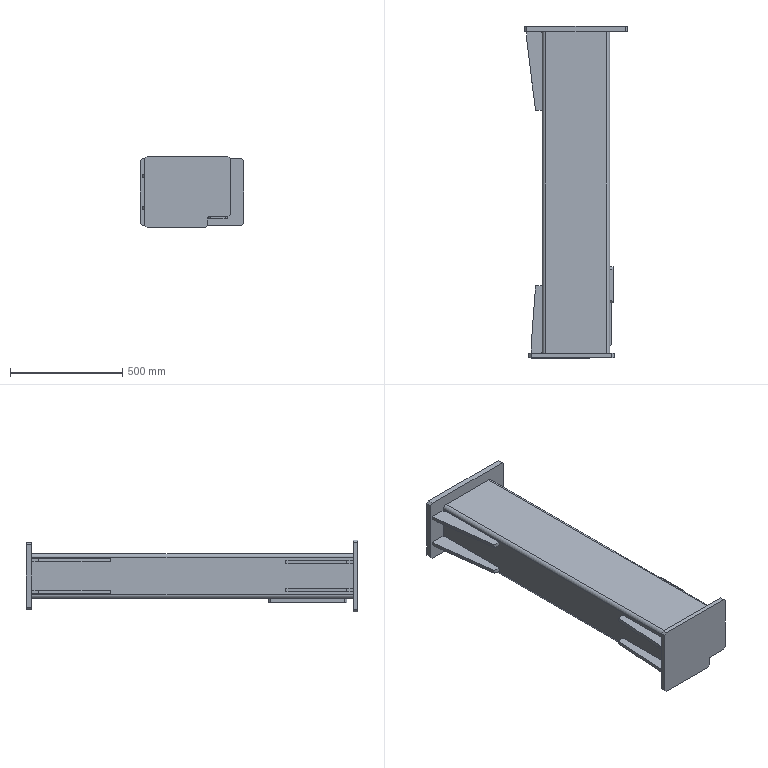Part | SolidWorks | features ICE 6, MirrorPattern 2, Extrusion 1 | 1 solid | 85 faces | box 460 x 1476 x 320 mm | volume 18498922 mm3 | plane 76 | cylinder 9 | commonest cylinder face diameters 16 x4 32 x4 10 x1